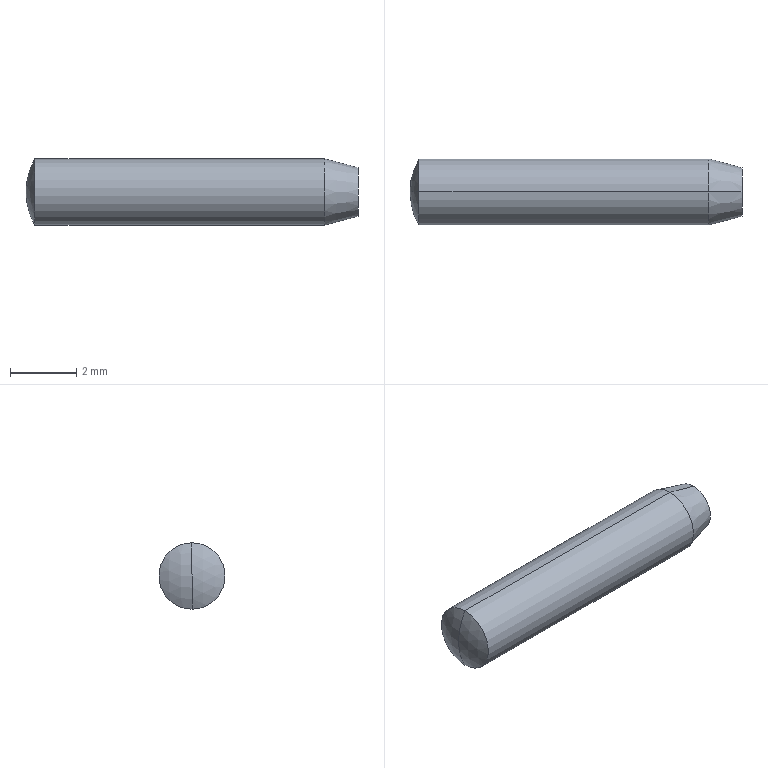Part | SolidWorks | features Revolution 1 | 1 solid | 7 faces | box 10 x 2 x 2 mm | volume 30.238 mm3 | cone 2 | cylinder 2 | sphere 2 | plane 1 | commonest cylinder face diameters 2 x2
STEP:
#1=CARTESIAN_POINT('',(0.,0.,0.7321));
#2=VERTEX_POINT('',#1);
#3=CARTESIAN_POINT('',(0.,0.,-0.7321));
#4=VERTEX_POINT('',#3);
#5=CARTESIAN_POINT('',(0.,0.,0.));
#6=DIRECTION('',(-1.,0.,0.));
#7=DIRECTION('',(0.,0.,1.));
#8=AXIS2_PLACEMENT_3D('',#5,#6,#7);
#9=CIRCLE('',#8,0.7321);
#10=EDGE_CURVE('',#2,#4,#9,.T.);
#11=ORIENTED_EDGE('',*,*,#10,.T.);
#12=CARTESIAN_POINT('',(-1.,0.,-1.));
#13=VERTEX_POINT('',#12);
#14=CARTESIAN_POINT('',(-1.,0.,-1.));
#15=DIRECTION('',(-0.9659,0.,-0.2588));
#16=VECTOR('',#15,1000.);
#17=LINE('',#14,#16);
#18=EDGE_CURVE('',#4,#13,#17,.T.);
#19=ORIENTED_EDGE('',*,*,#18,.T.);
#20=CARTESIAN_POINT('',(-1.,0.,1.));
#21=VERTEX_POINT('',#20);
#22=CARTESIAN_POINT('',(-1.,0.,0.));
#23=DIRECTION('',(-1.,0.,0.));
#24=DIRECTION('',(0.,0.,1.));
#25=AXIS2_PLACEMENT_3D('',#22,#23,#24);
#26=CIRCLE('',#25,1.);
#27=EDGE_CURVE('',#21,#13,#26,.T.);
#28=ORIENTED_EDGE('',*,*,#27,.F.);
#29=CARTESIAN_POINT('',(-1.,0.,1.));
#30=DIRECTION('',(-0.9659,0.,0.2588));
#31=VECTOR('',#30,1000.);
#32=LINE('',#29,#31);
#33=EDGE_CURVE('',#2,#21,#32,.T.);
#34=ORIENTED_EDGE('',*,*,#33,.F.);
#35=EDGE_LOOP('',(#11,#19,#28,#34));
#36=FACE_OUTER_BOUND('',#35,.T.);
#37=CARTESIAN_POINT('',(-1.,0.,0.));
#38=DIRECTION('',(-1.,0.,0.));
#39=DIRECTION('',(0.,0.,1.));
#40=AXIS2_PLACEMENT_3D('',#37,#38,#39);
#41=CONICAL_SURFACE('',#40,1.,0.2618);
#42=ADVANCED_FACE('',(#36),#41,.T.);
#43=ORIENTED_EDGE('',*,*,#27,.T.);
#44=CARTESIAN_POINT('',(-9.732,0.,-1.));
#45=VERTEX_POINT('',#44);
#46=CARTESIAN_POINT('',(-11.391,0.,-1.));
#47=DIRECTION('',(-1.,0.,0.));
#48=VECTOR('',#47,1000.);
#49=LINE('',#46,#48);
#50=EDGE_CURVE('',#13,#45,#49,.T.);
#51=ORIENTED_EDGE('',*,*,#50,.T.);
#52=CARTESIAN_POINT('',(-9.732,0.,1.));
#53=VERTEX_POINT('',#52);
#54=CARTESIAN_POINT('',(-9.732,0.,0.));
#55=DIRECTION('',(-1.,0.,0.));
#56=DIRECTION('',(0.,0.,1.));
#57=AXIS2_PLACEMENT_3D('',#54,#55,#56);
#58=CIRCLE('',#57,1.);
#59=EDGE_CURVE('',#53,#45,#58,.T.);
#60=ORIENTED_EDGE('',*,*,#59,.F.);
#61=CARTESIAN_POINT('',(-11.391,0.,1.));
#62=DIRECTION('',(-1.,0.,0.));
#63=VECTOR('',#62,1000.);
#64=LINE('',#61,#63);
#65=EDGE_CURVE('',#21,#53,#64,.T.);
#66=ORIENTED_EDGE('',*,*,#65,.F.);
#67=EDGE_LOOP('',(#43,#51,#60,#66));
#68=FACE_OUTER_BOUND('',#67,.T.);
#69=CARTESIAN_POINT('',(-11.391,0.,0.));
#70=DIRECTION('',(-1.,0.,0.));
#71=DIRECTION('',(0.,0.,1.));
#72=AXIS2_PLACEMENT_3D('',#69,#70,#71);
#73=CYLINDRICAL_SURFACE('',#72,1.);
#74=ADVANCED_FACE('',(#68),#73,.T.);
#75=CARTESIAN_POINT('',(-9.732,0.,0.));
#76=DIRECTION('',(-1.,0.,0.));
#77=DIRECTION('',(0.,0.,1.));
#78=AXIS2_PLACEMENT_3D('',#75,#76,#77);
#79=CIRCLE('',#78,1.);
#80=EDGE_CURVE('',#45,#53,#79,.T.);
#81=ORIENTED_EDGE('',*,*,#80,.T.);
#82=CARTESIAN_POINT('',(-10.,0.,0.));
#83=VERTEX_POINT('',#82);
#84=CARTESIAN_POINT('',(-8.,0.,0.));
#85=DIRECTION('',(0.,-1.,0.));
#86=DIRECTION('',(0.,0.,-1.));
#87=AXIS2_PLACEMENT_3D('',#84,#85,#86);
#88=CIRCLE('',#87,2.);
#89=EDGE_CURVE('',#53,#83,#88,.T.);
#90=ORIENTED_EDGE('',*,*,#89,.T.);
#91=CARTESIAN_POINT('',(-8.,0.,0.));
#92=DIRECTION('',(0.,1.,0.));
#93=DIRECTION('',(0.,0.,1.));
#94=AXIS2_PLACEMENT_3D('',#91,#92,#93);
#95=CIRCLE('',#94,2.);
#96=EDGE_CURVE('',#45,#83,#95,.T.);
#97=ORIENTED_EDGE('',*,*,#96,.F.);
#98=EDGE_LOOP('',(#81,#90,#97));
#99=FACE_OUTER_BOUND('',#98,.T.);
#100=CARTESIAN_POINT('',(-8.,0.,0.));
#101=DIRECTION('',(0.,-1.,0.));
#102=DIRECTION('',(0.,0.,-1.));
#103=AXIS2_PLACEMENT_3D('',#100,#101,#102);
#104=SPHERICAL_SURFACE('',#103,2.);
#105=ADVANCED_FACE('',(#99),#104,.T.);
#106=ORIENTED_EDGE('',*,*,#10,.F.);
#107=CARTESIAN_POINT('',(0.,0.,0.));
#108=DIRECTION('',(-1.,0.,0.));
#109=DIRECTION('',(0.,0.,1.));
#110=AXIS2_PLACEMENT_3D('',#107,#108,#109);
#111=CIRCLE('',#110,0.7321);
#112=EDGE_CURVE('',#4,#2,#111,.T.);
#113=ORIENTED_EDGE('',*,*,#112,.F.);
#114=EDGE_LOOP('',(#106,#113));
#115=FACE_OUTER_BOUND('',#114,.T.);
#116=CARTESIAN_POINT('',(0.,0.,0.));
#117=DIRECTION('',(1.,0.,0.));
#118=DIRECTION('',(0.,0.,-1.));
#119=AXIS2_PLACEMENT_3D('',#116,#117,#118);
#120=PLANE('',#119);
#121=ADVANCED_FACE('',(#115),#120,.T.);
#122=ORIENTED_EDGE('',*,*,#89,.F.);
#123=ORIENTED_EDGE('',*,*,#59,.T.);
#124=ORIENTED_EDGE('',*,*,#96,.T.);
#125=EDGE_LOOP('',(#122,#123,#124));
#126=FACE_OUTER_BOUND('',#125,.T.);
#127=CARTESIAN_POINT('',(-8.,0.,0.));
#128=DIRECTION('',(0.,-1.,0.));
#129=DIRECTION('',(0.,0.,-1.));
#130=AXIS2_PLACEMENT_3D('',#127,#128,#129);
#131=SPHERICAL_SURFACE('',#130,2.);
#132=ADVANCED_FACE('',(#126),#131,.T.);
#133=ORIENTED_EDGE('',*,*,#50,.F.);
#134=CARTESIAN_POINT('',(-1.,0.,0.));
#135=DIRECTION('',(-1.,0.,0.));
#136=DIRECTION('',(0.,0.,1.));
#137=AXIS2_PLACEMENT_3D('',#134,#135,#136);
#138=CIRCLE('',#137,1.);
#139=EDGE_CURVE('',#13,#21,#138,.T.);
#140=ORIENTED_EDGE('',*,*,#139,.T.);
#141=ORIENTED_EDGE('',*,*,#65,.T.);
#142=ORIENTED_EDGE('',*,*,#80,.F.);
#143=EDGE_LOOP('',(#133,#140,#141,#142));
#144=FACE_OUTER_BOUND('',#143,.T.);
#145=CARTESIAN_POINT('',(-11.391,0.,0.));
#146=DIRECTION('',(-1.,0.,0.));
#147=DIRECTION('',(0.,0.,1.));
#148=AXIS2_PLACEMENT_3D('',#145,#146,#147);
#149=CYLINDRICAL_SURFACE('',#148,1.);
#150=ADVANCED_FACE('',(#144),#149,.T.);
#151=ORIENTED_EDGE('',*,*,#18,.F.);
#152=ORIENTED_EDGE('',*,*,#112,.T.);
#153=ORIENTED_EDGE('',*,*,#33,.T.);
#154=ORIENTED_EDGE('',*,*,#139,.F.);
#155=EDGE_LOOP('',(#151,#152,#153,#154));
#156=FACE_OUTER_BOUND('',#155,.T.);
#157=CARTESIAN_POINT('',(-1.,0.,0.));
#158=DIRECTION('',(-1.,0.,0.));
#159=DIRECTION('',(0.,0.,1.));
#160=AXIS2_PLACEMENT_3D('',#157,#158,#159);
#161=CONICAL_SURFACE('',#160,1.,0.2618);
#162=ADVANCED_FACE('',(#156),#161,.T.);
#163=CLOSED_SHELL('',(#42,#74,#105,#121,#132,#150,#162));
#164=MANIFOLD_SOLID_BREP('',#163);
#165=CARTESIAN_POINT('',(0.,0.,0.));
#166=DIRECTION('',(0.,0.,1.));
#167=DIRECTION('',(1.,0.,0.));
#168=AXIS2_PLACEMENT_3D('',#165,#166,#167);
#169=(LENGTH_UNIT()NAMED_UNIT(*)SI_UNIT(.MILLI.,.METRE.));
#170=UNCERTAINTY_MEASURE_WITH_UNIT(LENGTH_MEASURE(0.00001),#169,'','');
#171=(NAMED_UNIT(*)PLANE_ANGLE_UNIT()SI_UNIT($,.RADIAN.));
#172=(NAMED_UNIT(*)SI_UNIT($,.STERADIAN.)SOLID_ANGLE_UNIT());
#173=(GEOMETRIC_REPRESENTATION_CONTEXT(3)GLOBAL_UNCERTAINTY_ASSIGNED_CONTEXT((#170))GLOBAL_UNIT_ASSIGNED_CONTEXT((#169,#171,#172))REPRESENTATION_CONTEXT('',''));
#174=ADVANCED_BREP_SHAPE_REPRESENTATION('',(#164,#168),#173);